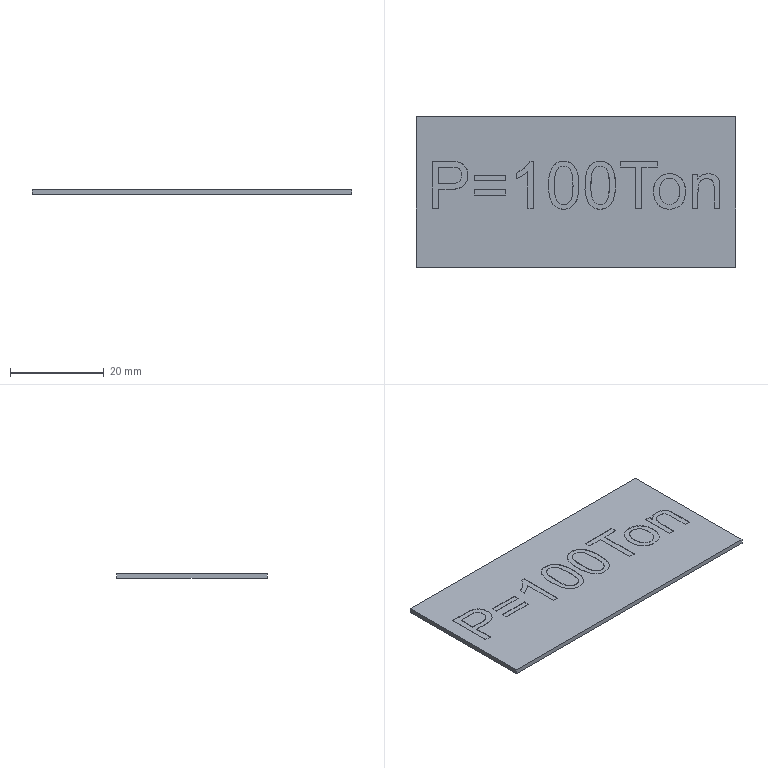Part | STEP file | lll_id1022_x_t | 1 solid | 70 faces | box 68.033 x 31.95 x 1 mm | volume 2155 mm3 | plane 49 | other 21